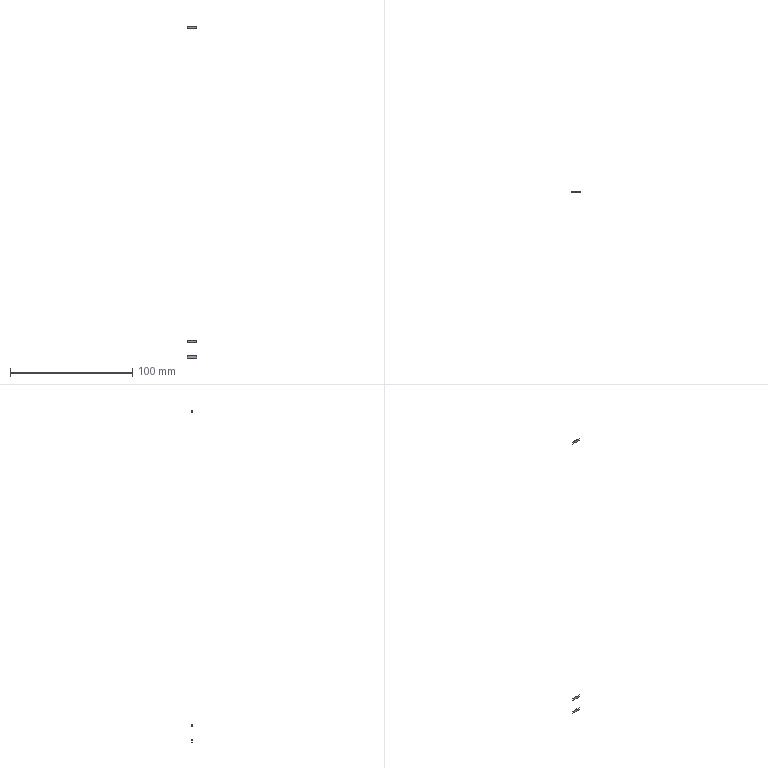Part | STEP file | ASND-0110-Q1-01-2 | 3 solids | 12 faces | box 7.937 x 0.5 x 271.8 mm | volume 14.332 mm3 | plane 9 | cylinder 3 | commonest cylinder face diameters 32 x3
STEP:
#1=CARTESIAN_POINT('',(0.,0.,0.));
#2=DIRECTION('',(0.,0.,1.));
#3=DIRECTION('',(1.,0.,0.));
#4=AXIS2_PLACEMENT_3D('',#1,#2,#3);
#5=CARTESIAN_POINT('',(-3.969,15.5,-142.3));
#6=VERTEX_POINT('',#5);
#7=CARTESIAN_POINT('',(3.969,15.5,-142.3));
#8=VERTEX_POINT('',#7);
#9=CARTESIAN_POINT('',(0.,0.,-142.3));
#10=DIRECTION('',(0.,0.,-1.));
#11=DIRECTION('',(-1.,0.,0.));
#12=AXIS2_PLACEMENT_3D('',#9,#10,#11);
#13=CIRCLE('',#12,16.);
#14=CARTESIAN_POINT('',(0.,14.,-142.3));
#15=DIRECTION('',(0.,0.,-1.));
#16=DIRECTION('',(0.7071,0.7071,0.));
#17=AXIS2_PLACEMENT_3D('',#14,#15,#16);
#18=PLANE('',#17);
#19=CARTESIAN_POINT('',(-9.899,9.899));
#20=DIRECTION('',(-0.7071,-0.7071));
#21=AXIS2_PLACEMENT_2D('',#19,#20);
#22=CIRCLE('',#21,16.);
#23=(GEOMETRIC_REPRESENTATION_CONTEXT(2)PARAMETRIC_REPRESENTATION_CONTEXT()REPRESENTATION_CONTEXT('',''));
#24=DEFINITIONAL_REPRESENTATION('',(#22),#23);
#25=PCURVE('',#18,#24);
#26=CARTESIAN_POINT('',(0.,0.,-141.4));
#27=DIRECTION('',(0.,0.,-1.));
#28=DIRECTION('',(-1.,0.,0.));
#29=AXIS2_PLACEMENT_3D('',#26,#27,#28);
#30=CYLINDRICAL_SURFACE('',#29,16.);
#31=CARTESIAN_POINT('',(0.,0.9));
#32=DIRECTION('',(1.,0.));
#33=VECTOR('',#32,1.);
#34=LINE('',#31,#33);
#35=(GEOMETRIC_REPRESENTATION_CONTEXT(2)PARAMETRIC_REPRESENTATION_CONTEXT()REPRESENTATION_CONTEXT('',''));
#36=DEFINITIONAL_REPRESENTATION('',(#34),#35);
#37=PCURVE('',#30,#36);
#38=SURFACE_CURVE('',#13,(#25,#37),.PCURVE_S1.);
#39=EDGE_CURVE('',#6,#8,#38,.T.);
#40=ORIENTED_EDGE('',*,*,#39,.T.);
#41=CARTESIAN_POINT('',(3.969,15.5,-142.3));
#42=DIRECTION('',(-1.,0.,0.));
#43=VECTOR('',#42,1.);
#44=LINE('',#41,#43);
#45=CARTESIAN_POINT('',(3.867,1.746));
#46=DIRECTION('',(-0.7071,-0.7071));
#47=VECTOR('',#46,1.);
#48=LINE('',#45,#47);
#49=(GEOMETRIC_REPRESENTATION_CONTEXT(2)PARAMETRIC_REPRESENTATION_CONTEXT()REPRESENTATION_CONTEXT('',''));
#50=DEFINITIONAL_REPRESENTATION('',(#48),#49);
#51=PCURVE('',#18,#50);
#52=CARTESIAN_POINT('',(0.,15.5,0.));
#53=DIRECTION('',(0.,-1.,0.));
#54=DIRECTION('',(0.7071,0.,0.7071));
#55=AXIS2_PLACEMENT_3D('',#52,#53,#54);
#56=PLANE('',#55);
#57=CARTESIAN_POINT('',(-97.815,-103.428));
#58=DIRECTION('',(-0.7071,0.7071));
#59=VECTOR('',#58,1.);
#60=LINE('',#57,#59);
#61=(GEOMETRIC_REPRESENTATION_CONTEXT(2)PARAMETRIC_REPRESENTATION_CONTEXT()REPRESENTATION_CONTEXT('',''));
#62=DEFINITIONAL_REPRESENTATION('',(#60),#61);
#63=PCURVE('',#56,#62);
#64=SURFACE_CURVE('',#44,(#51,#63),.PCURVE_S1.);
#65=EDGE_CURVE('',#8,#6,#64,.T.);
#66=ORIENTED_EDGE('',*,*,#65,.T.);
#67=EDGE_LOOP('',(#40,#66));
#68=FACE_BOUND('',#67,.T.);
#69=ADVANCED_FACE('',(#68),#18,.T.);
#70=ORIENTED_EDGE('',*,*,#39,.F.);
#71=CARTESIAN_POINT('',(-3.969,15.5,-140.5));
#72=VERTEX_POINT('',#71);
#73=CARTESIAN_POINT('',(-3.969,15.5,-140.5));
#74=DIRECTION('',(0.,0.,1.));
#75=VECTOR('',#74,1.);
#76=LINE('',#73,#75);
#77=CARTESIAN_POINT('',(1.32,-0.9));
#78=DIRECTION('',(0.,-1.));
#79=VECTOR('',#78,1.);
#80=LINE('',#77,#79);
#81=(GEOMETRIC_REPRESENTATION_CONTEXT(2)PARAMETRIC_REPRESENTATION_CONTEXT()REPRESENTATION_CONTEXT('',''));
#82=DEFINITIONAL_REPRESENTATION('',(#80),#81);
#83=PCURVE('',#30,#82);
#84=CARTESIAN_POINT('',(-102.155,-96.542));
#85=DIRECTION('',(0.7071,0.7071));
#86=VECTOR('',#85,1.);
#87=LINE('',#84,#86);
#88=(GEOMETRIC_REPRESENTATION_CONTEXT(2)PARAMETRIC_REPRESENTATION_CONTEXT()REPRESENTATION_CONTEXT('',''));
#89=DEFINITIONAL_REPRESENTATION('',(#87),#88);
#90=PCURVE('',#56,#89);
#91=SURFACE_CURVE('',#76,(#83,#90),.PCURVE_S1.);
#92=EDGE_CURVE('',#6,#72,#91,.T.);
#93=ORIENTED_EDGE('',*,*,#92,.T.);
#94=CARTESIAN_POINT('',(3.969,15.5,-140.5));
#95=VERTEX_POINT('',#94);
#96=CARTESIAN_POINT('',(0.,0.,-140.5));
#97=DIRECTION('',(0.,0.,-1.));
#98=DIRECTION('',(-1.,0.,0.));
#99=AXIS2_PLACEMENT_3D('',#96,#97,#98);
#100=CIRCLE('',#99,16.);
#101=CARTESIAN_POINT('',(0.,-0.9));
#102=DIRECTION('',(1.,0.));
#103=VECTOR('',#102,1.);
#104=LINE('',#101,#103);
#105=(GEOMETRIC_REPRESENTATION_CONTEXT(2)PARAMETRIC_REPRESENTATION_CONTEXT()REPRESENTATION_CONTEXT('',''));
#106=DEFINITIONAL_REPRESENTATION('',(#104),#105);
#107=PCURVE('',#30,#106);
#108=CARTESIAN_POINT('',(0.,15.75,-140.5));
#109=DIRECTION('',(0.,0.,1.));
#110=DIRECTION('',(0.7071,0.7071,0.));
#111=AXIS2_PLACEMENT_3D('',#108,#109,#110);
#112=PLANE('',#111);
#113=CARTESIAN_POINT('',(-22.451,0.1768));
#114=CARTESIAN_POINT('',(-2.855,19.773));
#115=CARTESIAN_POINT('',(4.318,-6.996));
#116=CARTESIAN_POINT('',(11.49,-33.764));
#117=CARTESIAN_POINT('',(-15.278,-26.592));
#118=CARTESIAN_POINT('',(-42.047,-19.419));
#119=CARTESIAN_POINT('',(-22.451,0.1768));
#120=(BOUNDED_CURVE()B_SPLINE_CURVE(2,(#113,#114,#115,#116,#117,#118,#119),.UNSPECIFIED.,.T.,.F.)B_SPLINE_CURVE_WITH_KNOTS((1,2,2,2,2,1),(-2.094,0.,2.094,4.189,6.283,8.378),.UNSPECIFIED.)CURVE()GEOMETRIC_REPRESENTATION_ITEM()RATIONAL_B_SPLINE_CURVE((1.,0.5,1.,0.5,1.,0.5,1.))REPRESENTATION_ITEM(''));
#121=(GEOMETRIC_REPRESENTATION_CONTEXT(2)PARAMETRIC_REPRESENTATION_CONTEXT()REPRESENTATION_CONTEXT('',''));
#122=DEFINITIONAL_REPRESENTATION('',(#120),#121);
#123=PCURVE('',#112,#122);
#124=SURFACE_CURVE('',#100,(#107,#123),.PCURVE_S1.);
#125=EDGE_CURVE('',#72,#95,#124,.T.);
#126=ORIENTED_EDGE('',*,*,#125,.T.);
#127=CARTESIAN_POINT('',(3.969,15.5,-140.5));
#128=DIRECTION('',(0.,0.,-1.));
#129=VECTOR('',#128,1.);
#130=LINE('',#127,#129);
#131=CARTESIAN_POINT('',(1.821,-0.9));
#132=DIRECTION('',(0.,1.));
#133=VECTOR('',#132,1.);
#134=LINE('',#131,#133);
#135=(GEOMETRIC_REPRESENTATION_CONTEXT(2)PARAMETRIC_REPRESENTATION_CONTEXT()REPRESENTATION_CONTEXT('',''));
#136=DEFINITIONAL_REPRESENTATION('',(#134),#135);
#137=PCURVE('',#30,#136);
#138=CARTESIAN_POINT('',(-96.542,-102.155));
#139=DIRECTION('',(-0.7071,-0.7071));
#140=VECTOR('',#139,1.);
#141=LINE('',#138,#140);
#142=(GEOMETRIC_REPRESENTATION_CONTEXT(2)PARAMETRIC_REPRESENTATION_CONTEXT()REPRESENTATION_CONTEXT('',''));
#143=DEFINITIONAL_REPRESENTATION('',(#141),#142);
#144=PCURVE('',#56,#143);
#145=SURFACE_CURVE('',#130,(#137,#144),.PCURVE_S1.);
#146=EDGE_CURVE('',#95,#8,#145,.T.);
#147=ORIENTED_EDGE('',*,*,#146,.T.);
#148=EDGE_LOOP('',(#70,#93,#126,#147));
#149=FACE_BOUND('',#148,.T.);
#150=ADVANCED_FACE('',(#149),#30,.T.);
#151=ORIENTED_EDGE('',*,*,#125,.F.);
#152=CARTESIAN_POINT('',(-3.969,15.5,-140.5));
#153=DIRECTION('',(1.,0.,0.));
#154=VECTOR('',#153,1.);
#155=LINE('',#152,#154);
#156=CARTESIAN_POINT('',(-2.983,2.629));
#157=DIRECTION('',(0.7071,-0.7071));
#158=VECTOR('',#157,1.);
#159=LINE('',#156,#158);
#160=(GEOMETRIC_REPRESENTATION_CONTEXT(2)PARAMETRIC_REPRESENTATION_CONTEXT()REPRESENTATION_CONTEXT('',''));
#161=DEFINITIONAL_REPRESENTATION('',(#159),#160);
#162=PCURVE('',#112,#161);
#163=CARTESIAN_POINT('',(-102.155,-96.542));
#164=DIRECTION('',(0.7071,-0.7071));
#165=VECTOR('',#164,1.);
#166=LINE('',#163,#165);
#167=(GEOMETRIC_REPRESENTATION_CONTEXT(2)PARAMETRIC_REPRESENTATION_CONTEXT()REPRESENTATION_CONTEXT('',''));
#168=DEFINITIONAL_REPRESENTATION('',(#166),#167);
#169=PCURVE('',#56,#168);
#170=SURFACE_CURVE('',#155,(#162,#169),.PCURVE_S1.);
#171=EDGE_CURVE('',#72,#95,#170,.T.);
#172=ORIENTED_EDGE('',*,*,#171,.T.);
#173=EDGE_LOOP('',(#151,#172));
#174=FACE_BOUND('',#173,.T.);
#175=ADVANCED_FACE('',(#174),#112,.T.);
#176=ORIENTED_EDGE('',*,*,#92,.F.);
#177=ORIENTED_EDGE('',*,*,#65,.F.);
#178=ORIENTED_EDGE('',*,*,#146,.F.);
#179=ORIENTED_EDGE('',*,*,#171,.F.);
#180=EDGE_LOOP('',(#176,#177,#178,#179));
#181=FACE_BOUND('',#180,.T.);
#182=ADVANCED_FACE('',(#181),#56,.T.);
#183=CLOSED_SHELL('',(#69,#150,#175,#182));
#184=MANIFOLD_SOLID_BREP('',#183);
#185=CARTESIAN_POINT('',(-3.969,15.5,-129.5));
#186=VERTEX_POINT('',#185);
#187=CARTESIAN_POINT('',(3.969,15.5,-129.5));
#188=VERTEX_POINT('',#187);
#189=CARTESIAN_POINT('',(0.,0.,-129.5));
#190=DIRECTION('',(0.,0.,-1.));
#191=DIRECTION('',(-1.,0.,0.));
#192=AXIS2_PLACEMENT_3D('',#189,#190,#191);
#193=CIRCLE('',#192,16.);
#194=CARTESIAN_POINT('',(0.,15.75,-129.5));
#195=DIRECTION('',(0.,0.,-1.));
#196=DIRECTION('',(0.7071,0.7071,0.));
#197=AXIS2_PLACEMENT_3D('',#194,#195,#196);
#198=PLANE('',#197);
#199=CARTESIAN_POINT('',(-11.137,11.137));
#200=DIRECTION('',(-0.7071,-0.7071));
#201=AXIS2_PLACEMENT_2D('',#199,#200);
#202=CIRCLE('',#201,16.);
#203=(GEOMETRIC_REPRESENTATION_CONTEXT(2)PARAMETRIC_REPRESENTATION_CONTEXT()REPRESENTATION_CONTEXT('',''));
#204=DEFINITIONAL_REPRESENTATION('',(#202),#203);
#205=PCURVE('',#198,#204);
#206=CARTESIAN_POINT('',(0.,0.,-128.6));
#207=DIRECTION('',(0.,0.,-1.));
#208=DIRECTION('',(-1.,0.,0.));
#209=AXIS2_PLACEMENT_3D('',#206,#207,#208);
#210=CYLINDRICAL_SURFACE('',#209,16.);
#211=CARTESIAN_POINT('',(0.,0.9));
#212=DIRECTION('',(1.,0.));
#213=VECTOR('',#212,1.);
#214=LINE('',#211,#213);
#215=(GEOMETRIC_REPRESENTATION_CONTEXT(2)PARAMETRIC_REPRESENTATION_CONTEXT()REPRESENTATION_CONTEXT('',''));
#216=DEFINITIONAL_REPRESENTATION('',(#214),#215);
#217=PCURVE('',#210,#216);
#218=SURFACE_CURVE('',#193,(#205,#217),.PCURVE_S1.);
#219=EDGE_CURVE('',#186,#188,#218,.T.);
#220=ORIENTED_EDGE('',*,*,#219,.T.);
#221=CARTESIAN_POINT('',(3.969,15.5,-129.5));
#222=DIRECTION('',(-1.,0.,0.));
#223=VECTOR('',#222,1.);
#224=LINE('',#221,#223);
#225=CARTESIAN_POINT('',(2.629,2.983));
#226=DIRECTION('',(-0.7071,-0.7071));
#227=VECTOR('',#226,1.);
#228=LINE('',#225,#227);
#229=(GEOMETRIC_REPRESENTATION_CONTEXT(2)PARAMETRIC_REPRESENTATION_CONTEXT()REPRESENTATION_CONTEXT('',''));
#230=DEFINITIONAL_REPRESENTATION('',(#228),#229);
#231=PCURVE('',#198,#230);
#232=CARTESIAN_POINT('',(0.,15.5,0.));
#233=DIRECTION('',(0.,-1.,0.));
#234=DIRECTION('',(0.7071,0.,0.7071));
#235=AXIS2_PLACEMENT_3D('',#232,#233,#234);
#236=PLANE('',#235);
#237=CARTESIAN_POINT('',(-88.764,-94.377));
#238=DIRECTION('',(-0.7071,0.7071));
#239=VECTOR('',#238,1.);
#240=LINE('',#237,#239);
#241=(GEOMETRIC_REPRESENTATION_CONTEXT(2)PARAMETRIC_REPRESENTATION_CONTEXT()REPRESENTATION_CONTEXT('',''));
#242=DEFINITIONAL_REPRESENTATION('',(#240),#241);
#243=PCURVE('',#236,#242);
#244=SURFACE_CURVE('',#224,(#231,#243),.PCURVE_S1.);
#245=EDGE_CURVE('',#188,#186,#244,.T.);
#246=ORIENTED_EDGE('',*,*,#245,.T.);
#247=EDGE_LOOP('',(#220,#246));
#248=FACE_BOUND('',#247,.T.);
#249=ADVANCED_FACE('',(#248),#198,.T.);
#250=ORIENTED_EDGE('',*,*,#219,.F.);
#251=CARTESIAN_POINT('',(-3.969,15.5,-127.7));
#252=VERTEX_POINT('',#251);
#253=CARTESIAN_POINT('',(-3.969,15.5,-127.7));
#254=DIRECTION('',(0.,0.,1.));
#255=VECTOR('',#254,1.);
#256=LINE('',#253,#255);
#257=CARTESIAN_POINT('',(1.32,-0.9));
#258=DIRECTION('',(0.,-1.));
#259=VECTOR('',#258,1.);
#260=LINE('',#257,#259);
#261=(GEOMETRIC_REPRESENTATION_CONTEXT(2)PARAMETRIC_REPRESENTATION_CONTEXT()REPRESENTATION_CONTEXT('',''));
#262=DEFINITIONAL_REPRESENTATION('',(#260),#261);
#263=PCURVE('',#210,#262);
#264=CARTESIAN_POINT('',(-93.104,-87.491));
#265=DIRECTION('',(0.7071,0.7071));
#266=VECTOR('',#265,1.);
#267=LINE('',#264,#266);
#268=(GEOMETRIC_REPRESENTATION_CONTEXT(2)PARAMETRIC_REPRESENTATION_CONTEXT()REPRESENTATION_CONTEXT('',''));
#269=DEFINITIONAL_REPRESENTATION('',(#267),#268);
#270=PCURVE('',#236,#269);
#271=SURFACE_CURVE('',#256,(#263,#270),.PCURVE_S1.);
#272=EDGE_CURVE('',#186,#252,#271,.T.);
#273=ORIENTED_EDGE('',*,*,#272,.T.);
#274=CARTESIAN_POINT('',(3.969,15.5,-127.7));
#275=VERTEX_POINT('',#274);
#276=CARTESIAN_POINT('',(0.,0.,-127.7));
#277=DIRECTION('',(0.,0.,-1.));
#278=DIRECTION('',(-1.,0.,0.));
#279=AXIS2_PLACEMENT_3D('',#276,#277,#278);
#280=CIRCLE('',#279,16.);
#281=CARTESIAN_POINT('',(0.,-0.9));
#282=DIRECTION('',(1.,0.));
#283=VECTOR('',#282,1.);
#284=LINE('',#281,#283);
#285=(GEOMETRIC_REPRESENTATION_CONTEXT(2)PARAMETRIC_REPRESENTATION_CONTEXT()REPRESENTATION_CONTEXT('',''));
#286=DEFINITIONAL_REPRESENTATION('',(#284),#285);
#287=PCURVE('',#210,#286);
#288=CARTESIAN_POINT('',(0.,14.,-127.7));
#289=DIRECTION('',(0.,0.,1.));
#290=DIRECTION('',(0.7071,0.7071,0.));
#291=AXIS2_PLACEMENT_3D('',#288,#289,#290);
#292=PLANE('',#291);
#293=CARTESIAN_POINT('',(-21.213,1.414));
#294=CARTESIAN_POINT('',(-1.617,21.01));
#295=CARTESIAN_POINT('',(5.555,-5.758));
#296=CARTESIAN_POINT('',(12.728,-32.527));
#297=CARTESIAN_POINT('',(-14.041,-25.354));
#298=CARTESIAN_POINT('',(-40.809,-18.182));
#299=CARTESIAN_POINT('',(-21.213,1.414));
#300=(BOUNDED_CURVE()B_SPLINE_CURVE(2,(#293,#294,#295,#296,#297,#298,#299),.UNSPECIFIED.,.T.,.F.)B_SPLINE_CURVE_WITH_KNOTS((1,2,2,2,2,1),(-2.094,0.,2.094,4.189,6.283,8.378),.UNSPECIFIED.)CURVE()GEOMETRIC_REPRESENTATION_ITEM()RATIONAL_B_SPLINE_CURVE((1.,0.5,1.,0.5,1.,0.5,1.))REPRESENTATION_ITEM(''));
#301=(GEOMETRIC_REPRESENTATION_CONTEXT(2)PARAMETRIC_REPRESENTATION_CONTEXT()REPRESENTATION_CONTEXT('',''));
#302=DEFINITIONAL_REPRESENTATION('',(#300),#301);
#303=PCURVE('',#292,#302);
#304=SURFACE_CURVE('',#280,(#287,#303),.PCURVE_S1.);
#305=EDGE_CURVE('',#252,#275,#304,.T.);
#306=ORIENTED_EDGE('',*,*,#305,.T.);
#307=CARTESIAN_POINT('',(3.969,15.5,-127.7));
#308=DIRECTION('',(0.,0.,-1.));
#309=VECTOR('',#308,1.);
#310=LINE('',#307,#309);
#311=CARTESIAN_POINT('',(1.821,-0.9));
#312=DIRECTION('',(0.,1.));
#313=VECTOR('',#312,1.);
#314=LINE('',#311,#313);
#315=(GEOMETRIC_REPRESENTATION_CONTEXT(2)PARAMETRIC_REPRESENTATION_CONTEXT()REPRESENTATION_CONTEXT('',''));
#316=DEFINITIONAL_REPRESENTATION('',(#314),#315);
#317=PCURVE('',#210,#316);
#318=CARTESIAN_POINT('',(-87.491,-93.104));
#319=DIRECTION('',(-0.7071,-0.7071));
#320=VECTOR('',#319,1.);
#321=LINE('',#318,#320);
#322=(GEOMETRIC_REPRESENTATION_CONTEXT(2)PARAMETRIC_REPRESENTATION_CONTEXT()REPRESENTATION_CONTEXT('',''));
#323=DEFINITIONAL_REPRESENTATION('',(#321),#322);
#324=PCURVE('',#236,#323);
#325=SURFACE_CURVE('',#310,(#317,#324),.PCURVE_S1.);
#326=EDGE_CURVE('',#275,#188,#325,.T.);
#327=ORIENTED_EDGE('',*,*,#326,.T.);
#328=EDGE_LOOP('',(#250,#273,#306,#327));
#329=FACE_BOUND('',#328,.T.);
#330=ADVANCED_FACE('',(#329),#210,.T.);
#331=ORIENTED_EDGE('',*,*,#305,.F.);
#332=CARTESIAN_POINT('',(-3.969,15.5,-127.7));
#333=DIRECTION('',(1.,0.,0.));
#334=VECTOR('',#333,1.);
#335=LINE('',#332,#334);
#336=CARTESIAN_POINT('',(-1.746,3.867));
#337=DIRECTION('',(0.7071,-0.7071));
#338=VECTOR('',#337,1.);
#339=LINE('',#336,#338);
#340=(GEOMETRIC_REPRESENTATION_CONTEXT(2)PARAMETRIC_REPRESENTATION_CONTEXT()REPRESENTATION_CONTEXT('',''));
#341=DEFINITIONAL_REPRESENTATION('',(#339),#340);
#342=PCURVE('',#292,#341);
#343=CARTESIAN_POINT('',(-93.104,-87.491));
#344=DIRECTION('',(0.7071,-0.7071));
#345=VECTOR('',#344,1.);
#346=LINE('',#343,#345);
#347=(GEOMETRIC_REPRESENTATION_CONTEXT(2)PARAMETRIC_REPRESENTATION_CONTEXT()REPRESENTATION_CONTEXT('',''));
#348=DEFINITIONAL_REPRESENTATION('',(#346),#347);
#349=PCURVE('',#236,#348);
#350=SURFACE_CURVE('',#335,(#342,#349),.PCURVE_S1.);
#351=EDGE_CURVE('',#252,#275,#350,.T.);
#352=ORIENTED_EDGE('',*,*,#351,.T.);
#353=EDGE_LOOP('',(#331,#352));
#354=FACE_BOUND('',#353,.T.);
#355=ADVANCED_FACE('',(#354),#292,.T.);
#356=ORIENTED_EDGE('',*,*,#326,.F.);
#357=ORIENTED_EDGE('',*,*,#351,.F.);
#358=ORIENTED_EDGE('',*,*,#272,.F.);
#359=ORIENTED_EDGE('',*,*,#245,.F.);
#360=EDGE_LOOP('',(#356,#357,#358,#359));
#361=FACE_BOUND('',#360,.T.);
#362=ADVANCED_FACE('',(#361),#236,.T.);
#363=CLOSED_SHELL('',(#249,#330,#355,#362));
#364=MANIFOLD_SOLID_BREP('',#363);
#365=CARTESIAN_POINT('',(-3.969,15.5,127.7));
#366=VERTEX_POINT('',#365);
#367=CARTESIAN_POINT('',(3.969,15.5,127.7));
#368=VERTEX_POINT('',#367);
#369=CARTESIAN_POINT('',(0.,0.,127.7));
#370=DIRECTION('',(0.,0.,-1.));
#371=DIRECTION('',(-1.,0.,0.));
#372=AXIS2_PLACEMENT_3D('',#369,#370,#371);
#373=CIRCLE('',#372,16.);
#374=CARTESIAN_POINT('',(0.,14.,127.7));
#375=DIRECTION('',(0.,0.,-1.));
#376=DIRECTION('',(0.7071,0.7071,0.));
#377=AXIS2_PLACEMENT_3D('',#374,#375,#376);
#378=PLANE('',#377);
#379=CARTESIAN_POINT('',(-9.899,9.899));
#380=DIRECTION('',(-0.7071,-0.7071));
#381=AXIS2_PLACEMENT_2D('',#379,#380);
#382=CIRCLE('',#381,16.);
#383=(GEOMETRIC_REPRESENTATION_CONTEXT(2)PARAMETRIC_REPRESENTATION_CONTEXT()REPRESENTATION_CONTEXT('',''));
#384=DEFINITIONAL_REPRESENTATION('',(#382),#383);
#385=PCURVE('',#378,#384);
#386=CARTESIAN_POINT('',(0.,0.,128.6));
#387=DIRECTION('',(0.,0.,-1.));
#388=DIRECTION('',(-1.,0.,0.));
#389=AXIS2_PLACEMENT_3D('',#386,#387,#388);
#390=CYLINDRICAL_SURFACE('',#389,16.);
#391=CARTESIAN_POINT('',(0.,0.9));
#392=DIRECTION('',(1.,0.));
#393=VECTOR('',#392,1.);
#394=LINE('',#391,#393);
#395=(GEOMETRIC_REPRESENTATION_CONTEXT(2)PARAMETRIC_REPRESENTATION_CONTEXT()REPRESENTATION_CONTEXT('',''));
#396=DEFINITIONAL_REPRESENTATION('',(#394),#395);
#397=PCURVE('',#390,#396);
#398=SURFACE_CURVE('',#373,(#385,#397),.PCURVE_S1.);
#399=EDGE_CURVE('',#366,#368,#398,.T.);
#400=ORIENTED_EDGE('',*,*,#399,.T.);
#401=CARTESIAN_POINT('',(3.969,15.5,127.7));
#402=DIRECTION('',(-1.,0.,0.));
#403=VECTOR('',#402,1.);
#404=LINE('',#401,#403);
#405=CARTESIAN_POINT('',(3.867,1.746));
#406=DIRECTION('',(-0.7071,-0.7071));
#407=VECTOR('',#406,1.);
#408=LINE('',#405,#407);
#409=(GEOMETRIC_REPRESENTATION_CONTEXT(2)PARAMETRIC_REPRESENTATION_CONTEXT()REPRESENTATION_CONTEXT('',''));
#410=DEFINITIONAL_REPRESENTATION('',(#408),#409);
#411=PCURVE('',#378,#410);
#412=CARTESIAN_POINT('',(0.,15.5,0.));
#413=DIRECTION('',(0.,-1.,0.));
#414=DIRECTION('',(0.7071,0.,0.7071));
#415=AXIS2_PLACEMENT_3D('',#412,#413,#414);
#416=PLANE('',#415);
#417=CARTESIAN_POINT('',(93.104,87.491));
#418=DIRECTION('',(-0.7071,0.7071));
#419=VECTOR('',#418,1.);
#420=LINE('',#417,#419);
#421=(GEOMETRIC_REPRESENTATION_CONTEXT(2)PARAMETRIC_REPRESENTATION_CONTEXT()REPRESENTATION_CONTEXT('',''));
#422=DEFINITIONAL_REPRESENTATION('',(#420),#421);
#423=PCURVE('',#416,#422);
#424=SURFACE_CURVE('',#404,(#411,#423),.PCURVE_S1.);
#425=EDGE_CURVE('',#368,#366,#424,.T.);
#426=ORIENTED_EDGE('',*,*,#425,.T.);
#427=EDGE_LOOP('',(#400,#426));
#428=FACE_BOUND('',#427,.T.);
#429=ADVANCED_FACE('',(#428),#378,.T.);
#430=ORIENTED_EDGE('',*,*,#399,.F.);
#431=CARTESIAN_POINT('',(-3.969,15.5,129.5));
#432=VERTEX_POINT('',#431);
#433=CARTESIAN_POINT('',(-3.969,15.5,129.5));
#434=DIRECTION('',(0.,0.,1.));
#435=VECTOR('',#434,1.);
#436=LINE('',#433,#435);
#437=CARTESIAN_POINT('',(1.32,-0.9));
#438=DIRECTION('',(0.,-1.));
#439=VECTOR('',#438,1.);
#440=LINE('',#437,#439);
#441=(GEOMETRIC_REPRESENTATION_CONTEXT(2)PARAMETRIC_REPRESENTATION_CONTEXT()REPRESENTATION_CONTEXT('',''));
#442=DEFINITIONAL_REPRESENTATION('',(#440),#441);
#443=PCURVE('',#390,#442);
#444=CARTESIAN_POINT('',(88.764,94.377));
#445=DIRECTION('',(0.7071,0.7071));
#446=VECTOR('',#445,1.);
#447=LINE('',#444,#446);
#448=(GEOMETRIC_REPRESENTATION_CONTEXT(2)PARAMETRIC_REPRESENTATION_CONTEXT()REPRESENTATION_CONTEXT('',''));
#449=DEFINITIONAL_REPRESENTATION('',(#447),#448);
#450=PCURVE('',#416,#449);
#451=SURFACE_CURVE('',#436,(#443,#450),.PCURVE_S1.);
#452=EDGE_CURVE('',#366,#432,#451,.T.);
#453=ORIENTED_EDGE('',*,*,#452,.T.);
#454=CARTESIAN_POINT('',(3.969,15.5,129.5));
#455=VERTEX_POINT('',#454);
#456=CARTESIAN_POINT('',(0.,0.,129.5));
#457=DIRECTION('',(0.,0.,-1.));
#458=DIRECTION('',(-1.,0.,0.));
#459=AXIS2_PLACEMENT_3D('',#456,#457,#458);
#460=CIRCLE('',#459,16.);
#461=CARTESIAN_POINT('',(0.,-0.9));
#462=DIRECTION('',(1.,0.));
#463=VECTOR('',#462,1.);
#464=LINE('',#461,#463);
#465=(GEOMETRIC_REPRESENTATION_CONTEXT(2)PARAMETRIC_REPRESENTATION_CONTEXT()REPRESENTATION_CONTEXT('',''));
#466=DEFINITIONAL_REPRESENTATION('',(#464),#465);
#467=PCURVE('',#390,#466);
#468=CARTESIAN_POINT('',(0.,15.75,129.5));
#469=DIRECTION('',(0.,0.,1.));
#470=DIRECTION('',(0.7071,0.7071,0.));
#471=AXIS2_PLACEMENT_3D('',#468,#469,#470);
#472=PLANE('',#471);
#473=CARTESIAN_POINT('',(-22.451,0.1768));
#474=CARTESIAN_POINT('',(-2.855,19.773));
#475=CARTESIAN_POINT('',(4.318,-6.996));
#476=CARTESIAN_POINT('',(11.49,-33.764));
#477=CARTESIAN_POINT('',(-15.278,-26.592));
#478=CARTESIAN_POINT('',(-42.047,-19.419));
#479=CARTESIAN_POINT('',(-22.451,0.1768));
#480=(BOUNDED_CURVE()B_SPLINE_CURVE(2,(#473,#474,#475,#476,#477,#478,#479),.UNSPECIFIED.,.T.,.F.)B_SPLINE_CURVE_WITH_KNOTS((1,2,2,2,2,1),(-2.094,0.,2.094,4.189,6.283,8.378),.UNSPECIFIED.)CURVE()GEOMETRIC_REPRESENTATION_ITEM()RATIONAL_B_SPLINE_CURVE((1.,0.5,1.,0.5,1.,0.5,1.))REPRESENTATION_ITEM(''));
#481=(GEOMETRIC_REPRESENTATION_CONTEXT(2)PARAMETRIC_REPRESENTATION_CONTEXT()REPRESENTATION_CONTEXT('',''));
#482=DEFINITIONAL_REPRESENTATION('',(#480),#481);
#483=PCURVE('',#472,#482);
#484=SURFACE_CURVE('',#460,(#467,#483),.PCURVE_S1.);
#485=EDGE_CURVE('',#432,#455,#484,.T.);
#486=ORIENTED_EDGE('',*,*,#485,.T.);
#487=CARTESIAN_POINT('',(3.969,15.5,129.5));
#488=DIRECTION('',(0.,0.,-1.));
#489=VECTOR('',#488,1.);
#490=LINE('',#487,#489);
#491=CARTESIAN_POINT('',(1.821,-0.9));
#492=DIRECTION('',(0.,1.));
#493=VECTOR('',#492,1.);
#494=LINE('',#491,#493);
#495=(GEOMETRIC_REPRESENTATION_CONTEXT(2)PARAMETRIC_REPRESENTATION_CONTEXT()REPRESENTATION_CONTEXT('',''));
#496=DEFINITIONAL_REPRESENTATION('',(#494),#495);
#497=PCURVE('',#390,#496);
#498=CARTESIAN_POINT('',(94.377,88.764));
#499=DIRECTION('',(-0.7071,-0.7071));
#500=VECTOR('',#499,1.);
#501=LINE('',#498,#500);
#502=(GEOMETRIC_REPRESENTATION_CONTEXT(2)PARAMETRIC_REPRESENTATION_CONTEXT()REPRESENTATION_CONTEXT('',''));
#503=DEFINITIONAL_REPRESENTATION('',(#501),#502);
#504=PCURVE('',#416,#503);
#505=SURFACE_CURVE('',#490,(#497,#504),.PCURVE_S1.);
#506=EDGE_CURVE('',#455,#368,#505,.T.);
#507=ORIENTED_EDGE('',*,*,#506,.T.);
#508=EDGE_LOOP('',(#430,#453,#486,#507));
#509=FACE_BOUND('',#508,.T.);
#510=ADVANCED_FACE('',(#509),#390,.T.);
#511=ORIENTED_EDGE('',*,*,#485,.F.);
#512=CARTESIAN_POINT('',(-3.969,15.5,129.5));
#513=DIRECTION('',(1.,0.,0.));
#514=VECTOR('',#513,1.);
#515=LINE('',#512,#514);
#516=CARTESIAN_POINT('',(-2.983,2.629));
#517=DIRECTION('',(0.7071,-0.7071));
#518=VECTOR('',#517,1.);
#519=LINE('',#516,#518);
#520=(GEOMETRIC_REPRESENTATION_CONTEXT(2)PARAMETRIC_REPRESENTATION_CONTEXT()REPRESENTATION_CONTEXT('',''));
#521=DEFINITIONAL_REPRESENTATION('',(#519),#520);
#522=PCURVE('',#472,#521);
#523=CARTESIAN_POINT('',(88.764,94.377));
#524=DIRECTION('',(0.7071,-0.7071));
#525=VECTOR('',#524,1.);
#526=LINE('',#523,#525);
#527=(GEOMETRIC_REPRESENTATION_CONTEXT(2)PARAMETRIC_REPRESENTATION_CONTEXT()REPRESENTATION_CONTEXT('',''));
#528=DEFINITIONAL_REPRESENTATION('',(#526),#527);
#529=PCURVE('',#416,#528);
#530=SURFACE_CURVE('',#515,(#522,#529),.PCURVE_S1.);
#531=EDGE_CURVE('',#432,#455,#530,.T.);
#532=ORIENTED_EDGE('',*,*,#531,.T.);
#533=EDGE_LOOP('',(#511,#532));
#534=FACE_BOUND('',#533,.T.);
#535=ADVANCED_FACE('',(#534),#472,.T.);
#536=ORIENTED_EDGE('',*,*,#452,.F.);
#537=ORIENTED_EDGE('',*,*,#425,.F.);
#538=ORIENTED_EDGE('',*,*,#506,.F.);
#539=ORIENTED_EDGE('',*,*,#531,.F.);
#540=EDGE_LOOP('',(#536,#537,#538,#539));
#541=FACE_BOUND('',#540,.T.);
#542=ADVANCED_FACE('',(#541),#416,.T.);
#543=CLOSED_SHELL('',(#429,#510,#535,#542));
#544=MANIFOLD_SOLID_BREP('',#543);
#545=(LENGTH_UNIT()NAMED_UNIT(*)SI_UNIT(.MILLI.,.METRE.));
#546=UNCERTAINTY_MEASURE_WITH_UNIT(LENGTH_MEASURE(0.0000001),#545,'','');
#547=(NAMED_UNIT(*)PLANE_ANGLE_UNIT()SI_UNIT($,.RADIAN.));
#548=(NAMED_UNIT(*)SI_UNIT($,.STERADIAN.)SOLID_ANGLE_UNIT());
#549=(GEOMETRIC_REPRESENTATION_CONTEXT(3)GLOBAL_UNCERTAINTY_ASSIGNED_CONTEXT((#546))GLOBAL_UNIT_ASSIGNED_CONTEXT((#545,#547,#548))REPRESENTATION_CONTEXT('',''));
#550=SHAPE_REPRESENTATION('',(#4,#184,#364,#544),#549);